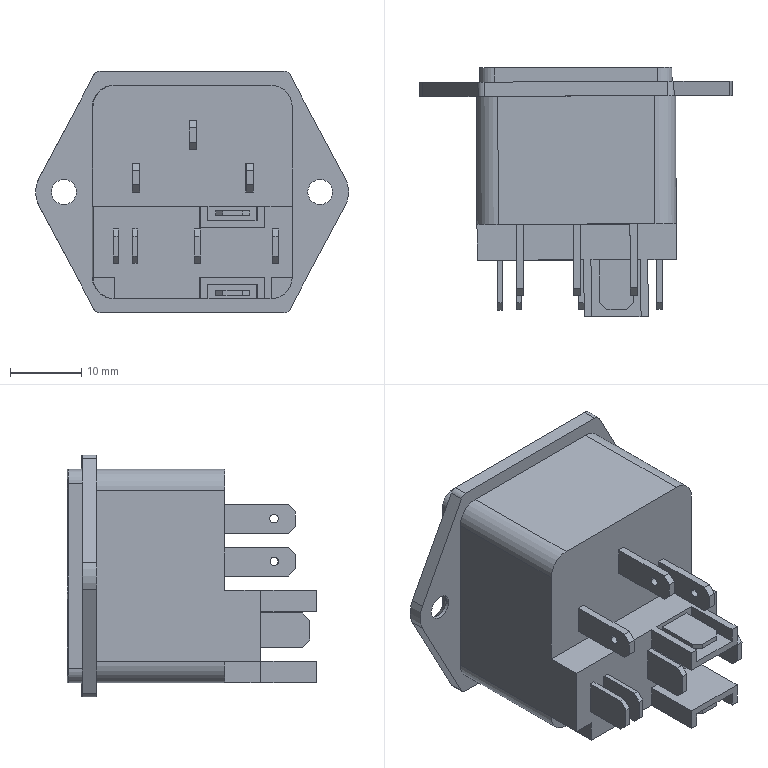Part | SolidWorks | features BaseBody 1 | 1 solid | 172 faces | box 44.008 x 35.054 x 34 mm | volume 10867 mm3 | plane 141 | cylinder 27 | cone 4 | commonest cylinder face diameters 1.2 x6 4 x6 2 x4 3.5 x4 6 x4 8 x3